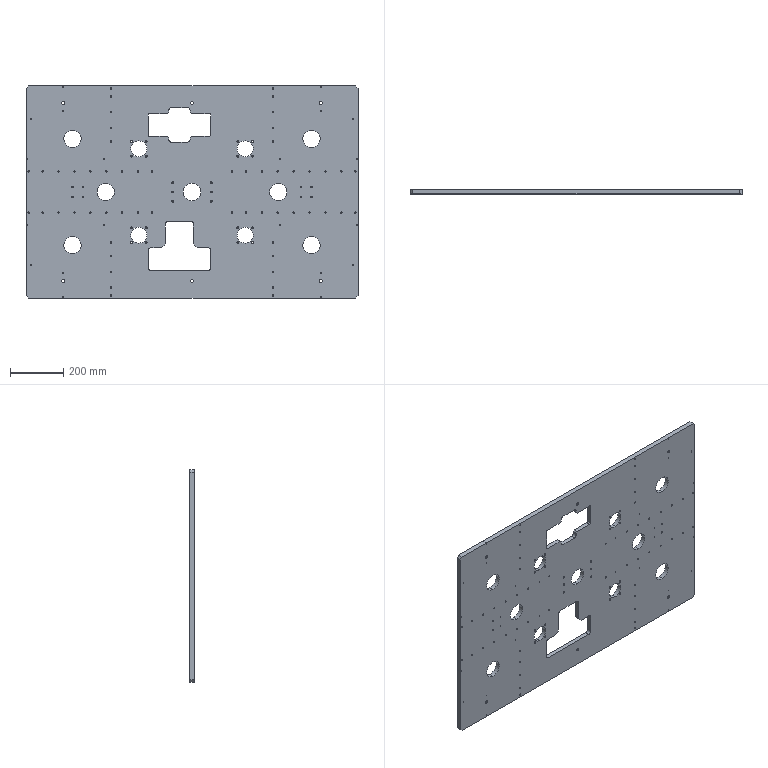Part | SolidWorks | features MirrorPattern 11, HoleWzd 10, LPattern 5, ICE 4, Chamfer 1, Extrusion 1 | 1 solid | 314 faces | box 1250 x 16 x 800 mm | volume 14520143 mm3 | cylinder 272 | plane 42 | commonest cylinder face diameters 5 x136 6.8 x44 3.3 x32 65 x14 11 x12 18 x12